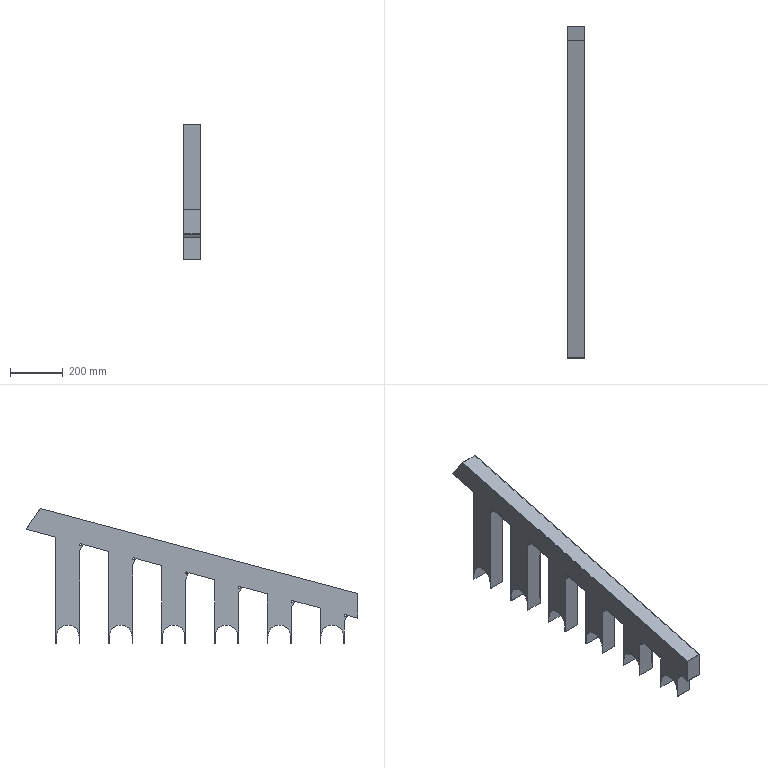Part | NX | features EXTRUDE 13, EXTRACT_STRING 12, Instance Feature 10, EXTRACT_FACE 6, DATUM_CSYS 3, Pattern Feature 2, SKETCH 2, DIVIDE_FACE 1, LINE 1, SHELL 1 | 1 solid | 107 faces | box 66 x 1255 x 510.77 mm | volume 1518508 mm3 | plane 83 | cylinder 24 | commonest cylinder face diameters 8 x12 86 x12